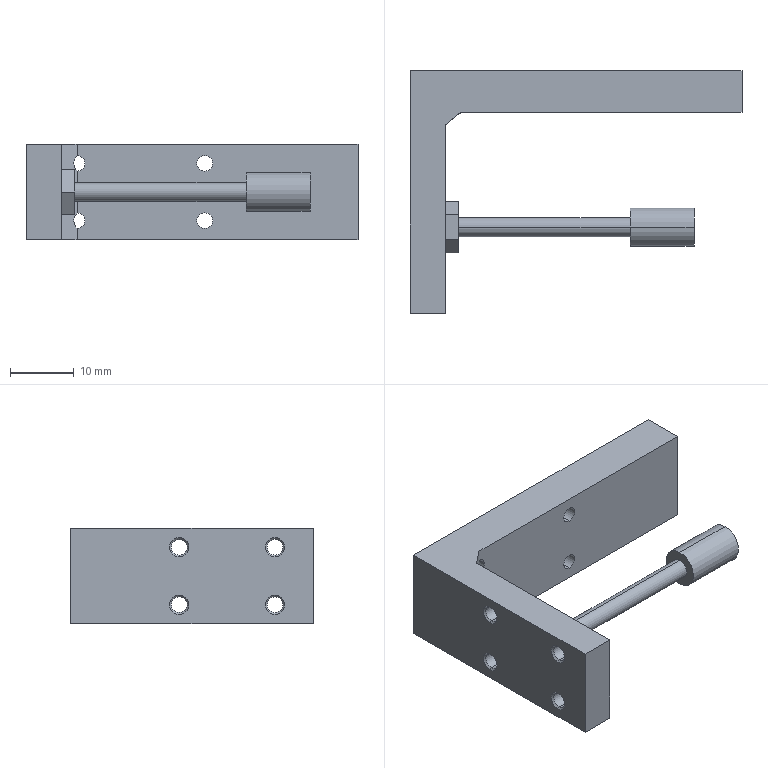Part | STEP file | MXH6-15-b | 1 solid | 56 faces | box 52 x 38 x 15 mm | volume 8036 mm3 | cylinder 20 | cone 18 | plane 18 | commonest cylinder face diameters 2.459 x16 3 x2 6 x2